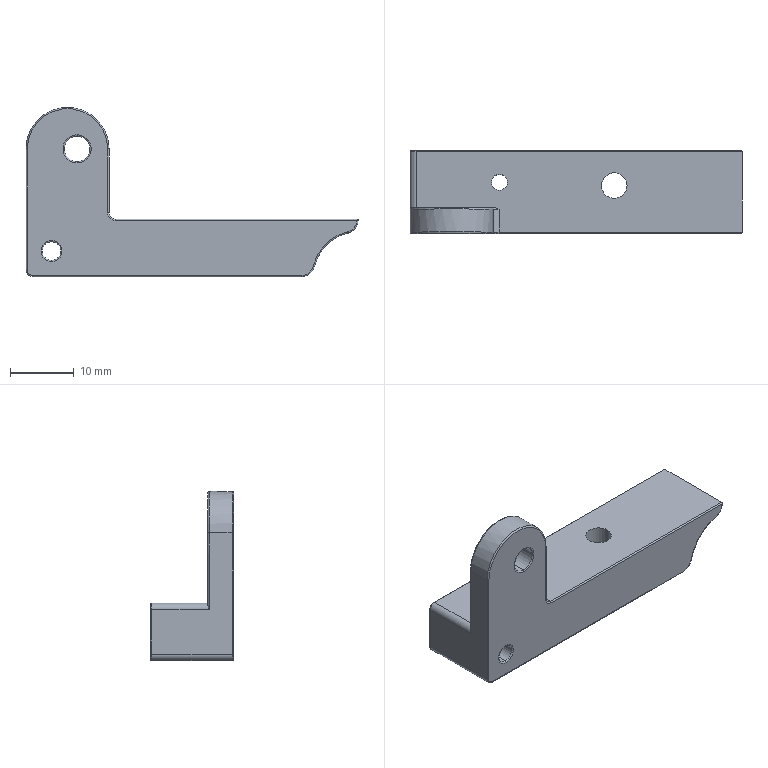Part | SolidWorks | features Fillet 2, ICE 2, Extrusion 1, HoleWzd 1 | 1 solid | 61 faces | box 52 x 13 x 26.5 mm | volume 6060 mm3 | cylinder 28 | torus 24 | plane 9 | commonest cylinder face diameters 0.4 x11 4 x6 2 x3 2.5 x2 2.9 x2 6 x2